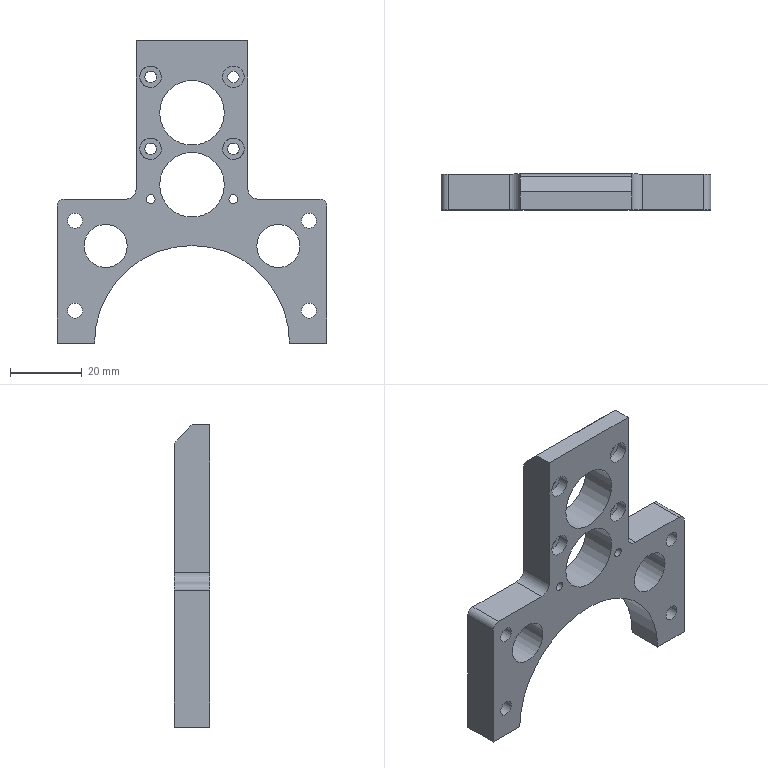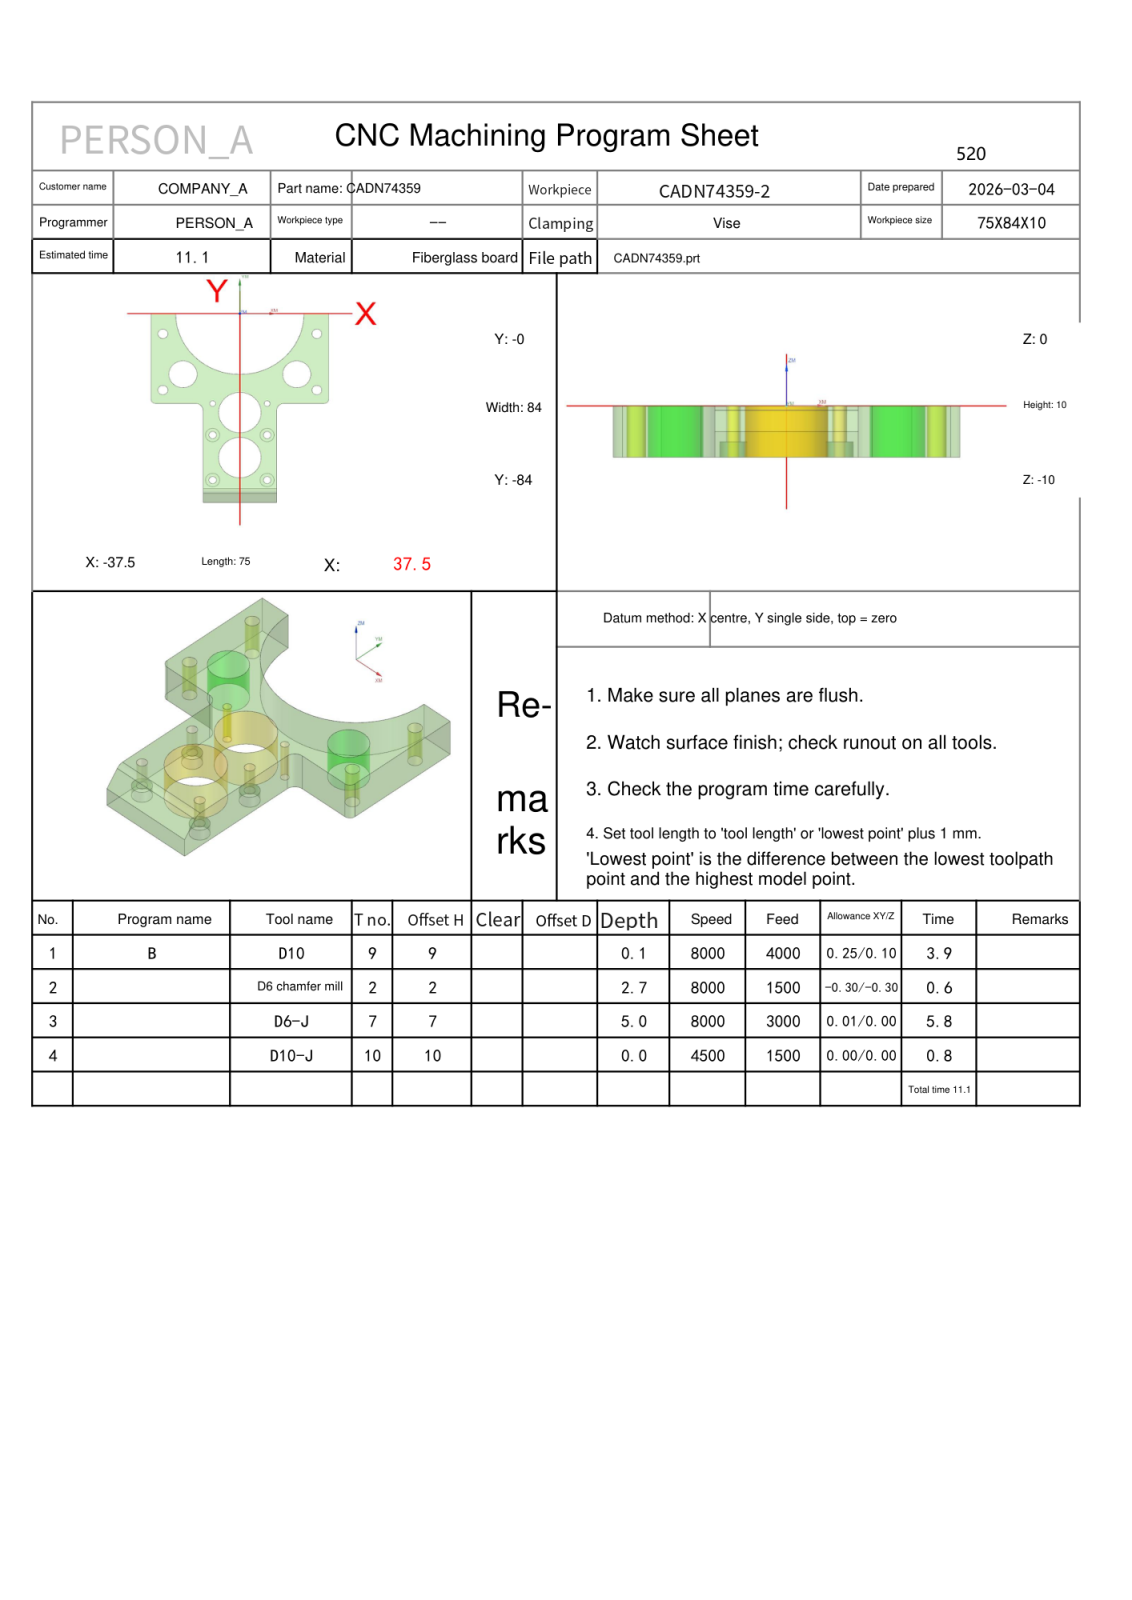NC program | NX | posted by the shop | part box 75 x 10 x 84 mm
Lines 1964 to 3114 of 5701:
N3 T07 M06
(D6-J  D=6. R=0. H=07 ce=0.01 di=0.00)
G00 G90 G54 X21.712 Y-80.94 M03 S8000
G43 H07 Z11.8
M08
Z.492
G01 Z-.008 F3000.
X16.602 Y-80.846
X16.57
G03 X16.121 Y-80.906 I0.0 J-1.715
G02 X15.515 Y-80.986 I-.606 J2.229
G01 X15.5
X-15.5
G03 X-15.879 Y-80.962 I-1.123 J-14.531
G01 X-16.055 Y-80.922
X-16.607 Y-80.838
X-16.608 Y-80.873 Z-.012
G03 X-15.5 Y-81.035 I2.245 J11.487
G01 X15.5
X16.055 Y-80.981
X16.161 Y-80.962
X16.401 Y-80.893
X16.602 Y-80.886
X16.601 Y-80.927 Z-.016
G03 X16.055 Y-81.021 I.066 J-2.018
G01 X15.5 Y-81.077
X-15.5
G02 X-16.607 Y-80.909 I.839 J9.286
G01 X-16.604 Y-80.941 Z-.02
X-16.448 Y-80.962
G03 X-15.5 Y-81.113 I1.334 J5.317
G01 X15.5
X16.055 Y-81.061
G02 X16.567 Y-80.964 I.512 J-1.302
G01 X16.6
Y-80.987 Z-.024
G03 X16.159 Y-81.048 I.009 J-1.695
G01 X16.141 Y-81.069
G02 X15.521 Y-81.146 I-.619 J2.438
G01 X15.5
X-15.5
G02 X-16.401 Y-80.994 I.166 J3.731
G01 X-16.601 Y-80.97
Y-80.994 Z-.028
X-16.401 Y-81.018
G03 X-15.5 Y-81.176 I.982 J2.937
G01 X15.5
G03 X16.401 Y-81.018 I-.152 J3.5
G01 X16.6 Y-81.01
Y-81.032 Z-.032
X16.519 Y-81.023
G03 X16.304 Y-81.088 I0.0 J-.393
G01 X16.247 Y-81.067
X16.187 Y-81.084
X16.149 Y-81.132
G02 X15.5 Y-81.204 I-.821 J4.412
G01 X-15.5
G02 X-16.401 Y-81.041 I.055 J2.868
G01 X-16.601 Y-81.015
X-16.602 Y-81.036 Z-.036
X-16.401 Y-81.064
G03 X-15.541 Y-81.231 I.86 J2.134
G01 X-15.5
X15.5
G03 X16.151 Y-81.154 I-.122 J3.839
G01 X16.192 Y-81.109
X16.252 Y-81.095
X16.308 Y-81.117
G02 X16.526 Y-81.046 I.218 J-.302
G01 X16.6 Y-81.054
Y-81.076 Z-.04
X16.53 Y-81.069
G03 X16.311 Y-81.143 I0.0 J-.364
G01 X16.266 Y-81.129
X16.222 Y-81.147
G02 X15.5 Y-81.256 I-.737 J2.434
G01 X-15.5
X-15.518
G02 X-16.401 Y-81.088 I0.0 J2.404
G01 X-16.602 Y-81.058
Y-81.075 Z-.042
Y-81.079 Z-.044
X-16.401 Y-81.111
G03 X-15.515 Y-81.279 I.885 J2.248
G01 X-15.5
X15.5
G03 X16.177 Y-81.189 I-.031 J2.811
G01 X16.24 Y-81.157
X16.264 Y-81.14
X16.293 Y-81.142
X16.313 Y-81.163
G02 X16.531 Y-81.092 I.218 J-.299
G01 X16.6 Y-81.098
Y-81.12 Z-.048
X16.533 Y-81.114
G03 X16.316 Y-81.183 I0.0 J-.376
G01 X16.23 Y-81.198
G02 X15.5 Y-81.302 I-.738 J2.563
G01 X-15.5
G02 X-16.24 Y-81.209 I.105 J3.832
G03 X-16.603 Y-81.1 I-.368 J-.568
G01 Y-81.118 Z-.05
Y-81.121 Z-.052
G02 X-16.269 Y-81.216 I-.017 J-.696
G03 X-15.503 Y-81.324 I.766 J2.672
G01 X-15.5
X15.5
X15.886 Y-81.297
G03 X16.318 Y-81.203 I-2.25 J11.35
G01 X16.401 Y-81.158
X16.6 Y-81.143
X16.601 Y-81.165 Z-.056
X16.401 Y-81.181
X16.321 Y-81.223
G02 X15.5 Y-81.344 I-.861 J2.99
G01 X-15.5
G02 X-16.273 Y-81.242 I.035 J3.244
G01 X-16.299 Y-81.228
G03 X-16.604 Y-81.142 I-.319 J-.551
G01 Y-81.159 Z-.058
Y-81.163 Z-.06
X-16.352 Y-81.22
X-16.302 Y-81.253
G03 X-15.5 Y-81.364 I.859 J3.258
G01 X15.5
X16.087 Y-81.306
X16.21 Y-81.279
G02 X16.601 Y-81.187 I.41 J-.865
G01 Y-81.209 Z-.064
X16.527 Y-81.196
X16.456 Y-81.22
X16.212 Y-81.298
X16.18 Y-81.306
X15.5 Y-81.384
X-15.5
G02 X-16.305 Y-81.274 I.128 J3.934
G01 X-16.355 Y-81.244
X-16.605 Y-81.185
Y-81.206 Z-.068
X-16.359 Y-81.267
X-16.334 Y-81.285
X-16.189 Y-81.321
X-15.5 Y-81.402
X15.5
X16.19 Y-81.32
X16.256 Y-81.306
X16.412 Y-81.257
X16.504 Y-81.226
X16.601 Y-81.231
Y-81.252 Z-.07
Y-81.253 Z-.072
X16.514 Y-81.246
X16.431 Y-81.273
X16.268 Y-81.32
X16.192 Y-81.336
X15.5 Y-81.421
X-15.5
G02 X-16.606 Y-81.227 I.282 J4.86
G01 Y-81.248 Z-.076
G03 X-15.5 Y-81.438 I1.428 J4.984
G01 X15.5
X16.055 Y-81.372
X16.193 Y-81.352
G02 X16.601 Y-81.276 I.536 J-1.722
G01 Y-81.294 Z-.08
G03 X16.195 Y-81.369 I.086 J-1.617
G01 X15.5 Y-81.456
X-15.5
G02 X-16.606 Y-81.266 I.383 J5.555
G01 X-16.604 Y-81.282 Z-.084
G03 X-15.5 Y-81.472 I1.502 J5.411
G01 X15.5
X16.197 Y-81.385
G02 X16.6 Y-81.308 I.462 J-1.326
G01 Y-81.328 Z-.088
X16.587
G03 X16.199 Y-81.401 I0.0 J-1.078
G01 X15.5 Y-81.489
X-15.5
G02 X-16.602 Y-81.295 I.388 J5.454
G01 X-16.6 Y-81.305 Z-.092
X-16.276 Y-81.391
X-16.2 Y-81.417
X-15.5 Y-81.505
X15.5
X16.201 Y-81.417
G02 X16.589 Y-81.343 I.388 J-.983
G01 X16.6
Y-81.344 Z-.094
Y-81.357 Z-.096
X16.591
G03 X16.203 Y-81.433 I0.0 J-1.036
G01 X15.5 Y-81.52
X-15.5
X-16.202 Y-81.433
G03 X-16.603 Y-81.336 I-.573 J-1.492
G01 Y-81.351 Z-.1
G02 X-16.204 Y-81.449 I-.125 J-1.374
G01 X-15.5 Y-81.535
X15.5
X16.205 Y-81.449
G02 X16.592 Y-81.372 I.388 J-.939
G01 X16.6
Y-81.373 Z-.102
Y-81.386 Z-.104
X16.555 Y-81.385
G03 X16.309 Y-81.42 I0.0 J-.886
G01 X16.282 Y-81.457
X16.237 Y-81.461
X15.5 Y-81.55
X-15.5
X-16.206 Y-81.465
G03 X-16.603 Y-81.367 I-.486 J-1.11
G01 X-16.602 Y-81.382 Z-.108
G02 X-16.208 Y-81.48 I-.064 J-1.098
G01 X-15.5 Y-81.565
X15.5
X16.241 Y-81.476
X16.285 Y-81.471
X16.31 Y-81.434
G02 X16.551 Y-81.399 I.241 J-.83
G01 X16.6 Y-81.401
Y-81.403 Z-.11
Y-81.415 Z-.112
X16.548 Y-81.414
G03 X16.312 Y-81.447 I0.0 J-.843
G01 X16.29 Y-81.484
X16.248 Y-81.489
X15.5 Y-81.579
X-15.5
X-16.209 Y-81.493
G03 X-16.602 Y-81.398 I-.45 J-.992
G01 Y-81.413 Z-.116
G02 X-16.211 Y-81.506 I-.051 J-1.078
G01 X-15.5 Y-81.594
X15.5
X16.212 Y-81.506
X16.288 Y-81.488
X16.313 Y-81.461
G02 X16.544 Y-81.428 I.231 J-.79
G01 X16.6 Y-81.43
Y-81.433 Z-.118
Y-81.444 Z-.12
X16.541 Y-81.442
G03 X16.315 Y-81.474 I0.0 J-.803
G01 X16.29 Y-81.502
X16.213 Y-81.519
X15.5 Y-81.607
X-15.5
G02 X-16.212 Y-81.519 I.413 J6.268
G03 X-16.602 Y-81.428 I-.433 J-.977
G01 X-16.601 Y-81.444 Z-.124
X-16.562 Y-81.442
X-16.392 Y-81.471
X-16.214 Y-81.532
G03 X-15.5 Y-81.621 I.991 J5.059
G01 X15.5
X16.215 Y-81.532
X16.291 Y-81.515
X16.317 Y-81.488
G02 X16.537 Y-81.456 I.221 J-.753
G01 X16.6 Y-81.459
Y-81.473 Z-.128
X16.534 Y-81.47
G03 X16.318 Y-81.501 I0.0 J-.766
G01 X16.297 Y-81.536
X16.257 Y-81.54
X15.5 Y-81.634
X-15.5
G02 X-16.344 Y-81.505 I.076 J3.31
G01 X-16.401 Y-81.481
X-16.601 Y-81.459
Y-81.475 Z-.132
X-16.401 Y-81.495
X-16.346 Y-81.519
G03 X-15.5 Y-81.647 I.907 J3.126
G01 X15.5
X16.218 Y-81.558
X16.294 Y-81.54
X16.32 Y-81.515
G02 X16.531 Y-81.485 I.211 J-.718
G01 X16.6 Y-81.488
Y-81.502 Z-.136
X16.528 Y-81.499
G03 X16.322 Y-81.529 I0.0 J-.732
G01 X16.295 Y-81.552
G02 X15.5 Y-81.66 I-.884 J3.495
G01 X-15.5
G02 X-16.347 Y-81.533 I.041 J3.159
G01 X-16.401 Y-81.509
X-16.601 Y-81.49
Y-81.505 Z-.14
X-16.401 Y-81.522
X-16.349 Y-81.547
G03 X-15.5 Y-81.673 I.87 J2.947
G01 X15.5
G03 X16.297 Y-81.563 I-.081 J3.54
G01 X16.323 Y-81.542
G02 X16.526 Y-81.513 I.203 J-.686
G01 X16.6 Y-81.517
Y-81.531 Z-.144
X16.523 Y-81.527
G03 X16.325 Y-81.556 I0.0 J-.699
G01 X16.301 Y-81.584
X16.265 Y-81.587
G02 X15.5 Y-81.686 I-.873 J3.773
G01 X-15.5
G02 X-16.351 Y-81.562 I.025 J3.149
G01 X-16.401 Y-81.536
X-16.6 Y-81.521
Z-.146
Y-81.536 Z-.148
X-16.401 Y-81.55
X-16.352 Y-81.575
G03 X-15.5 Y-81.698 I.883 J3.095
G01 X15.5
G03 X16.3 Y-81.587 I-.054 J3.329
G01 X16.326 Y-81.569
X16.521 Y-81.541
X16.6 Y-81.546
Y-81.56 Z-.152
X16.518 Y-81.555
X16.328 Y-81.583
X16.301 Y-81.599
X16.225 Y-81.622
X16.096 Y-81.65
X15.5 Y-81.71
X-15.5
G02 X-16.354 Y-81.586 I.044 J3.308
G01 X-16.401 Y-81.564
X-16.6 Y-81.552
Y-81.555 Z-.154
Y-81.567 Z-.156
X-16.401 Y-81.578
X-16.355 Y-81.598
G03 X-15.5 Y-81.722 I.918 J3.318
G01 X15.521
G03 X16.303 Y-81.611 I0.0 J2.802
G01 X16.33 Y-81.596
X16.516 Y-81.569
X16.6 Y-81.575
Y-81.589 Z-.16
X16.535 Y-81.57
X16.468 Y-81.572
X16.405 Y-81.595
X16.308 Y-81.622
G02 X15.504 Y-81.734 I-.804 J2.828
G01 X-15.5
G02 X-16.356 Y-81.61 I.086 J3.602
G01 X-16.401 Y-81.592
X-16.6 Y-81.583
Y-81.599 Z-.164
X-16.401 Y-81.606
X-16.358 Y-81.622
G03 X-15.5 Y-81.747 I.972 J3.687
G01 X15.5
G03 X16.403 Y-81.608 I-.107 J3.713
G01 X16.467 Y-81.586
X16.535 Y-81.585
X16.6 Y-81.605
Y-81.62 Z-.169
X16.526 Y-81.616
X16.388 Y-81.631
G02 X15.5 Y-81.759 I-1.238 J5.462
G01 X-15.5
G02 X-16.359 Y-81.635 I.149 J4.068
G01 X-16.401 Y-81.621
X-16.6 Y-81.615
Y-81.632 Z-.173
X-16.401 Y-81.636
G03 X-15.5 Y-81.771 I1.08 J4.135
G01 X15.5
X16.055 Y-81.71
X16.167 Y-81.69
X16.35 Y-81.65
X16.507 Y-81.628
X16.6 Y-81.636
Y-81.651 Z-.177
X16.505 Y-81.646
X16.309 Y-81.669
X16.168 Y-81.701
X16.055 Y-81.721
X15.5 Y-81.784
X-15.5
G02 X-16.298 Y-81.671 I.154 J3.967
G03 X-16.507 Y-81.645 I-.209 J-.848
G01 X-16.6 Y-81.65
Y-81.66 Z-.18
Y-81.661 Z-.182
X-16.514 Y-81.657
G02 X-16.283 Y-81.685 I0.0 J-.964
G03 X-15.5 Y-81.796 I.939 J3.809
G01 X15.5
X16.055 Y-81.732
X16.169 Y-81.712
X16.237 Y-81.696
G02 X16.507 Y-81.658 I.27 J-.937
G01 X16.6 Y-81.663
Y-81.674 Z-.186
X16.507 Y-81.67
G03 X16.238 Y-81.707 I0.0 J-.988
G01 X16.171 Y-81.724
X16.055 Y-81.744
X15.5 Y-81.809
X-15.5
G02 X-16.278 Y-81.697 I.156 J3.86
G03 X-16.512 Y-81.668 I-.234 J-.941
G01 X-16.6 Y-81.672
Y-81.684 Z-.191
X-16.508 Y-81.68
G02 X-16.239 Y-81.718 I0.0 J-.964
G03 X-15.5 Y-81.821 I.89 J3.679
G01 X15.5
X16.055 Y-81.755
X16.172 Y-81.735
X16.239 Y-81.718
G02 X16.507 Y-81.681 I.268 J-.964
G01 X16.6 Y-81.686
Y-81.697 Z-.196
X16.507 Y-81.693
G03 X16.24 Y-81.729 I0.0 J-1.015
G01 X16.173 Y-81.747
X16.055 Y-81.767
X15.5 Y-81.834
X-15.5
G02 X-16.24 Y-81.729 I.149 J3.723
G03 X-16.508 Y-81.692 I-.268 J-.941
G01 X-16.6 Y-81.696
Y-81.708 Z-.201
X-16.508 Y-81.704
G02 X-16.241 Y-81.74 I0.0 J-.993
G03 X-15.5 Y-81.846 I.894 J3.612
G01 X15.5
X16.055 Y-81.779
X16.174 Y-81.759
X16.241 Y-81.74
G02 X16.508 Y-81.705 I.266 J-.996
G01 X16.6 Y-81.709
Y-81.722 Z-.206
X16.508 Y-81.718
G03 X16.243 Y-81.752 I0.0 J-1.047
G01 X16.176 Y-81.771
X16.055 Y-81.792
X15.5 Y-81.859
X-15.5
G02 X-16.243 Y-81.752 I.154 J3.695
G03 X-16.508 Y-81.716 I-.266 J-.974
G01 X-16.6 Y-81.72
Y-81.733 Z-.211
X-16.509 Y-81.729
G02 X-16.244 Y-81.763 I0.0 J-1.028
G03 X-15.5 Y-81.871 I.895 J3.545
G01 X15.5
X16.055 Y-81.804
X16.177 Y-81.783
X16.244 Y-81.763
G02 X16.508 Y-81.73 I.264 J-1.032
G01 X16.6 Y-81.734
Y-81.747 Z-.216
X16.509 Y-81.743
G03 X16.178 Y-81.796 I0.0 J-1.063
G01 X16.055 Y-81.817
X15.5 Y-81.884
X-15.5
G02 X-16.245 Y-81.775 I.145 J3.593
G03 X-16.509 Y-81.742 I-.264 J-1.013
G01 X-16.6 Y-81.745
Y-81.758 Z-.221
X-16.509 Y-81.754
G02 X-16.18 Y-81.808 I0.0 J-1.025
G01 X-15.5 Y-81.897
X15.5
X16.055 Y-81.83
X16.179 Y-81.808
X16.2 Y-81.802
G02 X16.504 Y-81.755 I.304 J-.963
G01 X16.6 Y-81.759
Y-81.772 Z-.226
X16.504 Y-81.768
G03 X16.181 Y-81.821 I0.0 J-1.003
G01 X16.055 Y-81.843
X15.5 Y-81.91
X-15.5
G02 X-16.248 Y-81.8 I.124 J3.432
G03 X-16.51 Y-81.768 I-.262 J-1.059
G01 X-16.6 Y-81.771
Y-81.785 Z-.231
X-16.51 Y-81.781
G02 X-16.249 Y-81.812 I0.0 J-1.116
G03 X-15.5 Y-81.922 I.858 J3.224
G01 X15.5
X16.055 Y-81.856
X16.188 Y-81.832
G02 X16.503 Y-81.781 I.314 J-.934
G01 X16.6 Y-81.786
Y-81.799 Z-.237
X16.502 Y-81.794
G03 X16.184 Y-81.848 I0.0 J-.97
G01 X16.055 Y-81.87
X15.5 Y-81.935
X-15.5
G02 X-16.25 Y-81.824 I.093 J3.227
G03 X-16.51 Y-81.794 I-.26 J-1.113
G01 X-16.6 Y-81.798
Y-81.812 Z-.242
X-16.5 Y-81.806
G02 X-16.185 Y-81.861 I0.0 J-.937
G03 X-15.5 Y-81.948 I.826 J3.767
G01 X15.5
X16.055 Y-81.884
X16.185 Y-81.861
G02 X16.497 Y-81.807 I.312 J-.873
G01 X16.6 Y-81.812
Y-81.826 Z-.248
X16.493 Y-81.82
G03 X16.186 Y-81.874 I0.0 J-.888
G01 X16.055 Y-81.897
X15.5 Y-81.961
X-15.5
G02 X-16.186 Y-81.874 I.118 J3.717
G03 X-16.496 Y-81.819 I-.31 J-.841
G01 X-16.6 Y-81.825
Y-81.839 Z-.253
X-16.492 Y-81.832
G02 X-16.188 Y-81.888 I0.0 J-.858
G03 X-15.5 Y-81.973 I.799 J3.627
G01 X15.5
X16.055 Y-81.911
X16.188 Y-81.888
G02 X16.49 Y-81.833 I.302 J-.796
G01 X16.6 Y-81.84
Y-81.854 Z-.256
Z-.259
X16.487 Y-81.846
G03 X16.189 Y-81.902 I0.0 J-.818
G01 X16.055 Y-81.925
X15.5 Y-81.986
X-15.5
G02 X-16.189 Y-81.902 I.085 J3.564
G03 X-16.489 Y-81.846 I-.299 J-.767
G01 X-16.6 Y-81.853
Y-81.867 Z-.262
Y-81.868 Z-.264
X-16.513 Y-81.865
G02 X-16.257 Y-81.89 I0.0 J-1.329
G01 X-16.191 Y-81.916
G03 X-15.5 Y-81.999 I.749 J3.329
G01 X15.5
X16.055 Y-81.94
X16.191 Y-81.916
X16.257 Y-81.89
G02 X16.513 Y-81.865 I.255 J-1.34
G01 X16.6 Y-81.868
Y-81.881 Z-.267
Y-81.882 Z-.27
X16.513 Y-81.88
G03 X16.259 Y-81.903 I0.0 J-1.414
G01 X16.192 Y-81.93
X16.055 Y-81.954
X15.5 Y-82.012
X-15.5
G02 X-16.192 Y-81.93 I.037 J3.302
G01 X-16.259 Y-81.903
G03 X-16.514 Y-81.879 I-.255 J-1.356
G01 X-16.6 Y-81.882
Y-81.895 Z-.273
Y-81.896 Z-.276
X-16.514 Y-81.894
G02 X-16.26 Y-81.916 I0.0 J-1.438
G01 X-16.194 Y-81.943
G03 X-15.5 Y-82.024 I.726 J3.198
G01 X15.5
G03 X16.194 Y-81.943 I-.037 J3.318
G01 X16.26 Y-81.916
G02 X16.514 Y-81.894 I.254 J-1.448
G01 X16.6 Y-81.897
Y-81.909 Z-.279
Y-81.911 Z-.282
X16.515 Y-81.909
G03 X16.261 Y-81.93 I0.0 J-1.532
G01 X16.195 Y-81.955
G02 X15.5 Y-82.036 I-.737 J3.267
G01 X-15.5
G02 X-16.195 Y-81.955 I.043 J3.363
G01 X-16.261 Y-81.93
G03 X-16.515 Y-81.908 I-.254 J-1.48
G01 X-16.6 Y-81.911
Y-81.923 Z-.285
Y-81.925 Z-.287
X-16.516 Y-81.923
G02 X-16.263 Y-81.943 I0.0 J-1.574
G01 X-16.196 Y-81.967
G03 X-15.5 Y-82.049 I.755 J3.413
G01 X15.5
G03 X16.196 Y-81.967 I-.053 J3.444
G01 X16.263 Y-81.943
G02 X16.516 Y-81.923 I.253 J-1.582
G01 X16.6 Y-81.925
Y-81.937 Z-.29
Y-81.94 Z-.293
X16.517 Y-81.938
G03 X16.264 Y-81.957 I0.0 J-1.682
G01 X16.197 Y-81.979
X16.13 Y-81.994
G02 X15.5 Y-82.061 I-.74 J3.978
G01 X-15.5
G02 X-16.13 Y-81.994 I.12 J4.132
G01 X-16.197 Y-81.979
G03 X-16.487 Y-81.933 I-.289 J-.89
G01 X-16.6 Y-81.94
Y-81.95 Z-.296
Y-81.954 Z-.299
X-16.517 Y-81.951
G02 X-16.252 Y-81.98 I0.0 J-1.244
G03 X-15.5 Y-82.073 I.88 J4.031
G01 X15.5
G03 X16.25 Y-81.98 I-.124 J4.084
G02 X16.516 Y-81.951 I.266 J-1.214
G01 X16.6 Y-81.954
Y-81.965 Z-.302
Y-81.969 Z-.305
X16.508 Y-81.966
G03 X16.199 Y-82.002 I0.0 J-1.363
G02 X15.5 Y-82.085 I-.832 J3.993
G01 X-15.5
G02 X-16.204 Y-81.999 I.108 J3.791
G03 X-16.508 Y-81.966 I-.304 J-1.389
G01 X-16.6 Y-81.969
Y-81.985 Z-.311
X-16.52 Y-81.983
G02 X-16.2 Y-82.012 I0.0 J-1.74
G03 X-15.5 Y-82.098 I.849 J4.045
G01 X15.5
G03 X16.2 Y-82.012 I-.143 J4.082
G02 X16.52 Y-81.983 I.319 J-1.711
G01 X16.6 Y-81.985
Y-81.995 Z-.314
Y-81.999 Z-.317
X16.506 Y-81.997
G03 X16.161 Y-82.032 I0.0 J-1.718
G02 X15.5 Y-82.11 I-.8 J3.9
G01 X-15.5
G02 X-16.161 Y-82.032 I.139 J3.978
G03 X-16.506 Y-81.997 I-.345 J-1.683
G01 X-16.6 Y-81.999
Y-82.01 Z-.321
Y-82.012 Z-.324
X-16.521 Y-82.011
G02 X-16.202 Y-82.034 I0.0 J-2.201
G01 X-16.117 Y-82.059
G03 X-15.5 Y-82.123 I1.206 J8.622
G01 X15.5
G03 X16.117 Y-82.059 I-.589 J8.686
G01 X16.202 Y-82.034
G02 X16.521 Y-82.011 I.319 J-2.178
G01 X16.6 Y-82.012
Y-82.025 Z-.327
Y-82.026 Z-.33
X16.525 Y-82.025
G03 X16.203 Y-82.045 I0.0 J-2.513
G01 X16.118 Y-82.071
G02 X15.5 Y-82.136 I-1.726 J13.577
G01 X-15.5
G02 X-16.118 Y-82.071 I1.108 J13.642
G01 X-16.203 Y-82.045
G03 X-16.525 Y-82.025 I-.321 J-2.492
G01 X-16.6 Y-82.026
Y-82.039 Z-.337
X-16.53
G02 X-16.204 Y-82.057 I0.0 J-2.945
G01 X-16.175 Y-82.079
X-16.139 Y-82.076
X-15.5 Y-82.148
X15.5
G03 X16.055 Y-82.086 I-.15 J3.824
G01 X16.108 Y-82.095
X16.16 Y-82.085
X16.204 Y-82.057
G02 X16.53 Y-82.039 I.325 J-2.927
G01 X16.6
Y-82.053 Z-.343
X16.205 Y-82.068
X16.161 Y-82.097
X16.108 Y-82.107
X16.055 Y-82.097
G02 X15.5 Y-82.161 I-.698 J3.651
G01 X-15.5
X-16.055 Y-82.097
X-16.121 Y-82.096
X-16.205 Y-82.068
X-16.6 Y-82.053
Y-82.067 Z-.35
X-16.207 Y-82.079
X-16.161 Y-82.109
X-16.108 Y-82.12
X-16.055 Y-82.109
G03 X-15.5 Y-82.173 I.69 J3.549
G01 X15.5
G03 X16.055 Y-82.109 I-.131 J3.582
G01 X16.108 Y-82.12
X16.161 Y-82.109
X16.207 Y-82.079
X16.6 Y-82.067
Y-82.081 Z-.357
X16.208 Y-82.091
X16.162 Y-82.122
X16.109 Y-82.132
X16.055 Y-82.122
G02 X15.5 Y-82.186 I-.685 J3.477
G01 X-15.5
G02 X-16.055 Y-82.122 I.132 J3.566
G01 X-16.109 Y-82.132
X-16.162 Y-82.122
X-16.208 Y-82.091
X-16.6 Y-82.081
Y-82.095 Z-.363
X-16.209 Y-82.103
X-16.163 Y-82.134
X-16.109 Y-82.145
X-16.055 Y-82.134
G03 X-15.5 Y-82.199 I.681 J3.429
G01 X15.5
G03 X16.055 Y-82.134 I-.124 J3.475
G01 X16.109 Y-82.145
X16.163 Y-82.134
X16.209 Y-82.103
X16.6 Y-82.095
Y-82.109 Z-.37
X16.21 Y-82.115
X16.164 Y-82.146
X16.11 Y-82.157
X16.055 Y-82.146
G02 X15.5 Y-82.211 I-.67 J3.323
G01 X-15.5
G02 X-16.055 Y-82.146 I.116 J3.4
G01 X-16.11 Y-82.157
X-16.164 Y-82.146
X-16.21 Y-82.115
X-16.6 Y-82.109
Y-82.124 Z-.377
X-16.211 Y-82.127
X-16.165 Y-82.158
X-16.11 Y-82.169
X-16.055 Y-82.159
G03 X-15.5 Y-82.224 I.661 J3.246
G01 X15.5
G03 X16.055 Y-82.159 I-.106 J3.314
G01 X16.11 Y-82.169
X16.165 Y-82.158
X16.211 Y-82.127
X16.6 Y-82.124
Y-82.138 Z-.384
X16.212 Y-82.139
X16.166 Y-82.17
X16.111 Y-82.182
X16.055 Y-82.171
G02 X15.5 Y-82.236 I-.661 J3.245
G01 X-15.5
G02 X-16.055 Y-82.171 I.096 J3.231
G01 X-16.111 Y-82.182
X-16.166 Y-82.17
X-16.212 Y-82.139
X-16.6 Y-82.138
Y-82.152 Z-.388
Y-82.153 Z-.391
X-16.213 Y-82.151
X-16.166 Y-82.183
X-16.111 Y-82.194
X-16.055 Y-82.184
G03 X-15.5 Y-82.249 I.641 J3.092
G01 X15.5
G03 X16.055 Y-82.184 I-.101 J3.284
G01 X16.111 Y-82.194
X16.166 Y-82.183
X16.213 Y-82.151
X16.6 Y-82.153
Y-82.164 Z-.395
Y-82.167 Z-.398
X16.214 Y-82.163
X16.167 Y-82.195
X16.111 Y-82.207
X16.055 Y-82.197
G02 X15.5 Y-82.261 I-.649 J3.175
G01 X-15.5
G02 X-16.055 Y-82.197 I.075 J3.079
G01 X-16.111 Y-82.207
X-16.167 Y-82.195
X-16.214 Y-82.163
X-16.6 Y-82.167
Y-82.175 Z-.402
Y-82.179 Z-.406
X-16.215 Y-82.176
X-16.168 Y-82.207
X-16.112 Y-82.219
X-16.055 Y-82.21
G03 X-15.5 Y-82.274 I.623 J2.978
G01 X15.5
G03 X16.055 Y-82.21 I-.083 J3.176
G01 X16.112 Y-82.219
X16.168 Y-82.207
X16.215 Y-82.176
X16.6 Y-82.179
Y-82.187 Z-.409
Y-82.191 Z-.413
X16.217 Y-82.188
X16.168 Y-82.219
X16.112 Y-82.231
X16.055 Y-82.223
G02 X15.5 Y-82.286 I-.625 J3.031
G01 X-15.5
G02 X-16.055 Y-82.223 I.058 J2.989
G01 X-16.112 Y-82.231
X-16.168 Y-82.219
X-16.217 Y-82.188
X-16.6 Y-82.191
Y-82.199 Z-.417
Y-82.203 Z-.42
X-16.218 Y-82.201
X-16.19 Y-82.227
X-16.152 Y-82.225
X-15.5 Y-82.299
X15.5
G03 X16.055 Y-82.236 I-.055 J3.004
G01 X16.113 Y-82.243
X16.169 Y-82.231
X16.218 Y-82.201
X16.6 Y-82.203
Y-82.211 Z-.424
Y-82.215 Z-.428
X16.219 Y-82.214
G02 X15.513 Y-82.311 I-.706 J2.517
G01 X15.5
X-15.5
X-15.513
G02 X-16.219 Y-82.214 I0.0 J2.614
G01 X-16.6 Y-82.215
Y-82.223 Z-.431
Y-82.227 Z-.435
X-16.22
G03 X-15.5 Y-82.323 I.739 J2.78
G01 X15.5
G03 X16.22 Y-82.227 I-.019 J2.876
G01 X16.6
Y-82.235 Z-.439
Y-82.24 Z-.443
X16.221
G02 X15.5 Y-82.336 I-.737 J2.786
G01 X-15.5
G02 X-16.221 Y-82.24 I.015 J2.876
G01 X-16.6
Y-82.248 Z-.446
Y-82.252 Z-.45
X-16.223 Y-82.253
G03 X-15.5 Y-82.348 I.723 J2.7
G01 X15.5
G03 X16.223 Y-82.253 I0.0 J2.793
G01 X16.6 Y-82.252
Y-82.26 Z-.454
Y-82.264 Z-.458
X16.224 Y-82.266
G02 X15.518 Y-82.36 I-.705 J2.596
G01 X15.5
X-15.5
X-15.516
G02 X-16.224 Y-82.266 I0.0 J2.71
G01 X-16.6 Y-82.264
Y-82.273 Z-.462
Y-82.277 Z-.465
X-16.225 Y-82.279
G03 X-15.511 Y-82.372 I.714 J2.698
G01 X-15.5
X15.5
X15.504
G03 X16.225 Y-82.279 I0.0 J2.841
G01 X16.6 Y-82.277
Y-82.285 Z-.469
Y-82.29 Z-.473
X16.226 Y-82.293
G02 X15.5 Y-82.385 I-.728 J2.845
G01 X-15.5
G02 X-16.226 Y-82.293 I.001 J2.928
G01 X-16.6 Y-82.29
Y-82.298 Z-.477
Y-82.302 Z-.481
X-16.228 Y-82.306
G03 X-15.5 Y-82.397 I.74 J2.986
G01 X15.5
G03 X16.228 Y-82.306 I-.012 J3.072
G01 X16.6 Y-82.302
Y-82.311 Z-.485
Y-82.315 Z-.489
X16.229 Y-82.32
G02 X15.5 Y-82.409 I-.755 J3.162
G01 X-15.5
G02 X-16.229 Y-82.32 I.028 J3.263
G01 X-16.6 Y-82.315
Y-82.324 Z-.493
Y-82.328 Z-.497
X-16.23 Y-82.334
G03 X-15.5 Y-82.421 I.774 J3.381
G01 X15.5
G03 X16.23 Y-82.334 I-.041 J3.444
G01 X16.6 Y-82.328
Y-82.336 Z-.501
Y-82.341 Z-.505
X16.223 Y-82.347
G02 X15.5 Y-82.433 I-.765 J3.386
G01 X-15.5
G02 X-16.223 Y-82.347 I.045 J3.5
G01 X-16.6 Y-82.341
Y-82.349 Z-.509
Y-82.353 Z-.512
X-16.225 Y-82.36
G03 X-15.5 Y-82.444 I.772 J3.47
G01 X15.5
G03 X16.225 Y-82.36 I-.048 J3.562
G01 X16.6 Y-82.353
Y-82.362 Z-.516
Y-82.366 Z-.52
X16.226 Y-82.372
G02 X15.5 Y-82.456 I-.779 J3.567
G01 X-15.5
G02 X-16.226 Y-82.372 I.062 J3.727
G01 X-16.6 Y-82.366
Y-82.375 Z-.524
Y-82.379 Z-.528
X-16.227 Y-82.385
G03 X-15.5 Y-82.468 I.807 J3.855
G01 X15.5
G03 X16.227 Y-82.385 I-.058 J3.743
G01 X16.6 Y-82.379
Y-82.388 Z-.532
Y-82.392 Z-.537
X16.228 Y-82.398
G02 X15.5 Y-82.48 I-.797 J3.823
G01 X-15.5
G02 X-16.228 Y-82.398 I.097 J4.154
G01 X-16.6 Y-82.393
Y-82.402 Z-.541
Y-82.406 Z-.545
X-16.229 Y-82.411
G03 X-15.5 Y-82.492 I.868 J4.524
G01 X15.5
G03 X16.229 Y-82.411 I-.085 J4.117
G01 X16.6 Y-82.406
Y-82.416 Z-.549
Y-82.42 Z-.553
X16.45 Y-82.415
G03 X16.055 Y-82.449 I0.0 J-2.288
G02 X15.514 Y-82.504 I-.542 J2.654
G01 X15.5 Y-82.503
X-15.5
G02 X-16.231 Y-82.424 I.181 J5.082
G01 X-16.6 Y-82.42
Y-82.429 Z-.558
Y-82.433 Z-.562
X-16.232 Y-82.438
G03 X-15.5 Y-82.515 I1.003 J5.973
G01 X15.5
X15.512
G03 X16. Y-82.471 I0.0 J2.684
G02 X16.454 Y-82.429 I.454 J-2.455
G01 X16.6 Y-82.433
Y-82.443 Z-.566
Y-82.447 Z-.57
X16.51 Y-82.446
G03 X16.055 Y-82.471 I0.0 J-4.182
G01 X15.949 Y-82.489
G02 X15.512 Y-82.527 I-.437 J2.504
G01 X-15.5
G02 X-15.935 Y-82.494 I.33 J7.084
G03 X-16.465 Y-82.444 I-.53 J-2.807
G01 X-16.6 Y-82.447
Y-82.457 Z-.575
Y-82.461 Z-.579
X-16.521 Y-82.46
G02 X-16.055 Y-82.482 I0.0 J-5.067
G01 X-15.935 Y-82.505
G03 X-15.5 Y-82.539 I.778 J7.046
G01 X15.506
G03 X15.948 Y-82.501 I0.0 J2.569
G01 X16.055 Y-82.482
G02 X16.523 Y-82.46 I.468 J-5.035
G01 X16.6 Y-82.461
Y-82.471 Z-.583
Y-82.475 Z-.588
X16.543
G03 X16.055 Y-82.493 I0.0 J-6.402
G01 X15.94 Y-82.513
G02 X15.507 Y-82.551 I-.433 J2.481
G01 X-15.5
G02 X-15.936 Y-82.516 I.343 J6.95
G01 X-16.055 Y-82.493
G03 X-16.539 Y-82.475 I-.484 J-6.41
G01 X-16.6
Y-82.485 Z-.592
Y-82.489 Z-.596
X-16.571
G02 X-16.055 Y-82.504 I0.0 J-8.801
G03 X-15.5 Y-82.563 I.664 J3.646
G01 X15.5
G03 X16.055 Y-82.505 I-.029 J2.959
G02 X16.576 Y-82.489 I.52 J-8.718
G01 X16.6
Y-82.503 Z-.605
G03 X16.055 Y-82.516 I.02 J-12.581
G02 X15.5 Y-82.574 I-.591 J2.949
G01 X-15.5
G02 X-16.055 Y-82.516 I.11 J3.693
G01 X-16.6 Y-82.503
Y-82.513 Z-.61
Y-82.516 Z-.614
X-16.554
G02 X-16.055 Y-82.527 I0.0 J-10.927
G03 X-15.5 Y-82.586 I.663 J3.598
G01 X15.5
G03 X16.055 Y-82.527 I-.041 J3.042
G02 X16.563 Y-82.515 I.507 J-10.76
G01 X16.6 Y-82.516
Y-82.526 Z-.623
X16.55
G03 X16.055 Y-82.539 I0.0 J-9.347
G02 X15.5 Y-82.598 I-.599 J3.004
G01 X-15.5
G02 X-16.055 Y-82.539 I.102 J3.599
G03 X-16.536 Y-82.526 I-.48 J-9.398
G01 X-16.6 Y-82.527
Y-82.537 Z-.632
X-16.155 Y-82.546
X-16.055 Y-82.55
G03 X-15.5 Y-82.609 I.65 J3.462
G01 X15.5
G03 X16.055 Y-82.551 I-.044 J3.068
G02 X16.541 Y-82.536 I.486 J-8.24
G01 X16.6 Y-82.537
Y-82.544 Z-.637
Y-82.547 Z-.641
X16.534
G03 X16.055 Y-82.562 I0.0 J-7.39
G02 X15.5 Y-82.621 I-.598 J3.
G01 X-15.5
G02 X-16.055 Y-82.562 I.083 J3.426
G01 X-16.156 Y-82.556
X-16.6 Y-82.548
Y-82.556 Z-.646
Y-82.559 Z-.65
X-16.493 Y-82.558
G02 X-16.055 Y-82.574 I0.0 J-6.295
G01 X-15.94 Y-82.595
G03 X-15.5 Y-82.632 I.579 J4.233
G01 X15.501
G03 X15.937 Y-82.595 I0.0 J2.534
G01 X16.055 Y-82.574
G02 X16.528 Y-82.557 I.472 J-6.672
G01 X16.6 Y-82.558
Y-82.565 Z-.655
Y-82.569 Z-.659
X16.523 Y-82.568
G03 X16.055 Y-82.586 I0.0 J-6.109
G01 X15.938 Y-82.606
G02 X15.505 Y-82.644 I-.433 J2.481
G01 X-15.5
G02 X-16.055 Y-82.585 I.056 J3.194
G01 X-16.158 Y-82.578
X-16.6 Y-82.57
Y-82.578 Z-.664
Y-82.581 Z-.669
X-16.159 Y-82.589
X-16.055 Y-82.597
G03 X-15.5 Y-82.655 I.595 J3.006
G01 X15.502
G03 X15.947 Y-82.617 I0.0 J2.586
G01 X16.055 Y-82.598
G02 X16.471 Y-82.577 I.416 J-4.21
G01 X16.6 Y-82.579
Y-82.587 Z-.673
Y-82.59 Z-.678
X16.471 Y-82.588
G03 X16.055 Y-82.61 I0.0 J-3.972
G01 X15.955 Y-82.627
G02 X15.5 Y-82.667 I-.455 J2.605
G01 X-15.5
G02 X-16.055 Y-82.609 I.022 J2.928
G01 X-16.16 Y-82.599
X-16.6 Y-82.593
Y-82.601 Z-.683
Y-82.604 Z-.687
X-16.161 Y-82.61
X-16.055 Y-82.621
X-15.999 Y-82.632
G03 X-15.502 Y-82.678 I.498 J2.654
G01 X15.508
G03 X15.956 Y-82.639 I0.0 J2.605
G01 X16.055 Y-82.622
G02 X16.47 Y-82.599 I.415 J-3.722
G01 X16.6 Y-82.601
Y-82.609 Z-.692
Y-82.612 Z-.697
X16.47 Y-82.61
G03 X15.888 Y-82.658 I0.0 J-3.541
G02 X15.507 Y-82.69 I-.381 J2.286
G01 X-15.5
X-15.512
G02 X-15.943 Y-82.654 I0.0 J2.677
G01 X-16.055 Y-82.634
X-16.162 Y-82.621
X-16.6 Y-82.615
X-16.599 Y-82.623 Z-.701
Y-82.627 Z-.706
X-16.25 Y-82.628
X-16.163 Y-82.632
G03 X-15.5 Y-82.701 I.746 J3.978
G01 X15.504
G03 X15.98 Y-82.659 I0.0 J2.766
G01 X16.055 Y-82.646
G02 X16.508 Y-82.622 I.453 J-4.24
G01 X16.6 Y-82.623
Y-82.631 Z-.711
Y-82.634 Z-.716
X16.507 Y-82.633
G03 X16.055 Y-82.659 I0.0 J-4.022
G01 X15.5 Y-82.712
X-15.5
G02 X-16.164 Y-82.643 I.097 J4.182
G01 X-16.251 Y-82.64
X-16.599 Y-82.638
Y-82.646 Z-.72
Y-82.65 Z-.725
X-16.252 Y-82.651
X-16.165 Y-82.655
X-16.055 Y-82.67
X-15.5 Y-82.723
X15.5
X16.175 Y-82.66
G02 X16.505 Y-82.644 I.331 J-3.52
G01 X16.599 Y-82.646
Y-82.653 Z-.73
Y-82.657 Z-.735
X16.507 Y-82.655
G03 X16.204 Y-82.669 I0.0 J-3.3
G01 X15.5 Y-82.734
X-15.5
X-16.166 Y-82.666
X-16.599 Y-82.661
Y-82.669 Z-.74
Y-82.673 Z-.744
X-16.167 Y-82.677
X-16.055 Y-82.694
X-15.5 Y-82.745
X15.5
X16.214 Y-82.68